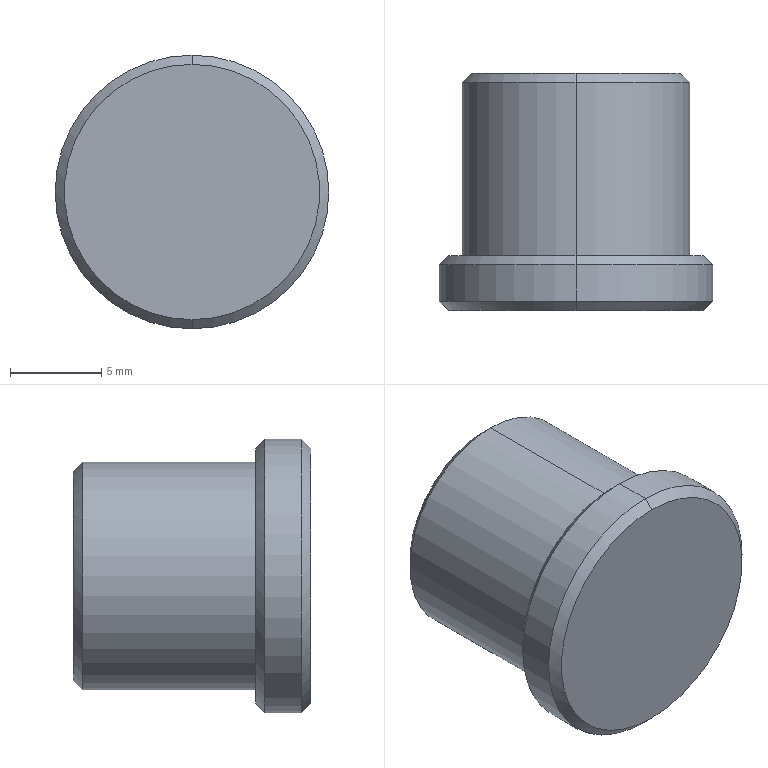Part | SolidWorks | features Chamfer 1, Revolution 1 | 1 solid | 13 faces | box 15 x 13 x 15 mm | volume 1741 mm3 | cone 6 | cylinder 4 | plane 3 | commonest cylinder face diameters 12.5 x2 15 x2
STEP:
#1=CARTESIAN_POINT('',(0.,13.,5.75));
#2=VERTEX_POINT('',#1);
#3=CARTESIAN_POINT('',(0.,13.,-5.75));
#4=VERTEX_POINT('',#3);
#5=CARTESIAN_POINT('',(0.,13.,0.));
#6=DIRECTION('',(0.,1.,0.));
#7=DIRECTION('',(0.,0.,1.));
#8=AXIS2_PLACEMENT_3D('',#5,#6,#7);
#9=CIRCLE('',#8,5.75);
#10=EDGE_CURVE('',#2,#4,#9,.T.);
#11=ORIENTED_EDGE('',*,*,#10,.F.);
#12=CARTESIAN_POINT('',(0.,12.5,6.25));
#13=VERTEX_POINT('',#12);
#14=CARTESIAN_POINT('',(0.,12.5,6.25));
#15=DIRECTION('',(0.,-0.7071,0.7071));
#16=VECTOR('',#15,1000.);
#17=LINE('',#14,#16);
#18=EDGE_CURVE('',#2,#13,#17,.T.);
#19=ORIENTED_EDGE('',*,*,#18,.T.);
#20=CARTESIAN_POINT('',(0.,12.5,-6.25));
#21=VERTEX_POINT('',#20);
#22=CARTESIAN_POINT('',(0.,12.5,0.));
#23=DIRECTION('',(0.,-1.,0.));
#24=DIRECTION('',(0.,0.,1.));
#25=AXIS2_PLACEMENT_3D('',#22,#23,#24);
#26=CIRCLE('',#25,6.25);
#27=EDGE_CURVE('',#21,#13,#26,.T.);
#28=ORIENTED_EDGE('',*,*,#27,.F.);
#29=CARTESIAN_POINT('',(0.,12.5,-6.25));
#30=DIRECTION('',(0.,-0.7071,-0.7071));
#31=VECTOR('',#30,1000.);
#32=LINE('',#29,#31);
#33=EDGE_CURVE('',#4,#21,#32,.T.);
#34=ORIENTED_EDGE('',*,*,#33,.F.);
#35=EDGE_LOOP('',(#11,#19,#28,#34));
#36=FACE_OUTER_BOUND('',#35,.T.);
#37=CARTESIAN_POINT('',(0.,12.5,0.));
#38=DIRECTION('',(0.,-1.,0.));
#39=DIRECTION('',(0.,0.,-1.));
#40=AXIS2_PLACEMENT_3D('',#37,#38,#39);
#41=CONICAL_SURFACE('',#40,6.25,0.7854);
#42=ADVANCED_FACE('',(#36),#41,.T.);
#43=CARTESIAN_POINT('',(0.,3.,7.));
#44=VERTEX_POINT('',#43);
#45=CARTESIAN_POINT('',(0.,3.,-7.));
#46=VERTEX_POINT('',#45);
#47=CARTESIAN_POINT('',(0.,3.,0.));
#48=DIRECTION('',(0.,1.,0.));
#49=DIRECTION('',(0.,0.,1.));
#50=AXIS2_PLACEMENT_3D('',#47,#48,#49);
#51=CIRCLE('',#50,7.);
#52=EDGE_CURVE('',#44,#46,#51,.T.);
#53=ORIENTED_EDGE('',*,*,#52,.F.);
#54=CARTESIAN_POINT('',(0.,2.5,7.5));
#55=VERTEX_POINT('',#54);
#56=CARTESIAN_POINT('',(0.,2.5,7.5));
#57=DIRECTION('',(0.,-0.7071,0.7071));
#58=VECTOR('',#57,1000.);
#59=LINE('',#56,#58);
#60=EDGE_CURVE('',#44,#55,#59,.T.);
#61=ORIENTED_EDGE('',*,*,#60,.T.);
#62=CARTESIAN_POINT('',(0.,2.5,-7.5));
#63=VERTEX_POINT('',#62);
#64=CARTESIAN_POINT('',(0.,2.5,0.));
#65=DIRECTION('',(0.,-1.,0.));
#66=DIRECTION('',(0.,0.,1.));
#67=AXIS2_PLACEMENT_3D('',#64,#65,#66);
#68=CIRCLE('',#67,7.5);
#69=EDGE_CURVE('',#63,#55,#68,.T.);
#70=ORIENTED_EDGE('',*,*,#69,.F.);
#71=CARTESIAN_POINT('',(0.,2.5,-7.5));
#72=DIRECTION('',(0.,-0.7071,-0.7071));
#73=VECTOR('',#72,1000.);
#74=LINE('',#71,#73);
#75=EDGE_CURVE('',#46,#63,#74,.T.);
#76=ORIENTED_EDGE('',*,*,#75,.F.);
#77=EDGE_LOOP('',(#53,#61,#70,#76));
#78=FACE_OUTER_BOUND('',#77,.T.);
#79=CARTESIAN_POINT('',(0.,2.5,0.));
#80=DIRECTION('',(0.,-1.,0.));
#81=DIRECTION('',(0.,0.,-1.));
#82=AXIS2_PLACEMENT_3D('',#79,#80,#81);
#83=CONICAL_SURFACE('',#82,7.5,0.7854);
#84=ADVANCED_FACE('',(#78),#83,.T.);
#85=CARTESIAN_POINT('',(0.,0.,-7.));
#86=VERTEX_POINT('',#85);
#87=CARTESIAN_POINT('',(0.,0.,7.));
#88=VERTEX_POINT('',#87);
#89=CARTESIAN_POINT('',(0.,0.,0.));
#90=DIRECTION('',(0.,-1.,0.));
#91=DIRECTION('',(0.,0.,-1.));
#92=AXIS2_PLACEMENT_3D('',#89,#90,#91);
#93=CIRCLE('',#92,7.);
#94=EDGE_CURVE('',#86,#88,#93,.T.);
#95=ORIENTED_EDGE('',*,*,#94,.F.);
#96=CARTESIAN_POINT('',(0.,0.5,-7.5));
#97=VERTEX_POINT('',#96);
#98=CARTESIAN_POINT('',(0.,0.,-7.));
#99=DIRECTION('',(0.,0.7071,-0.7071));
#100=VECTOR('',#99,1000.);
#101=LINE('',#98,#100);
#102=EDGE_CURVE('',#86,#97,#101,.T.);
#103=ORIENTED_EDGE('',*,*,#102,.T.);
#104=CARTESIAN_POINT('',(0.,0.5,7.5));
#105=VERTEX_POINT('',#104);
#106=CARTESIAN_POINT('',(0.,0.5,0.));
#107=DIRECTION('',(0.,1.,0.));
#108=DIRECTION('',(0.,0.,-1.));
#109=AXIS2_PLACEMENT_3D('',#106,#107,#108);
#110=CIRCLE('',#109,7.5);
#111=EDGE_CURVE('',#105,#97,#110,.T.);
#112=ORIENTED_EDGE('',*,*,#111,.F.);
#113=CARTESIAN_POINT('',(0.,0.,7.));
#114=DIRECTION('',(0.,0.7071,0.7071));
#115=VECTOR('',#114,1000.);
#116=LINE('',#113,#115);
#117=EDGE_CURVE('',#88,#105,#116,.T.);
#118=ORIENTED_EDGE('',*,*,#117,.F.);
#119=EDGE_LOOP('',(#95,#103,#112,#118));
#120=FACE_OUTER_BOUND('',#119,.T.);
#121=CARTESIAN_POINT('',(0.,0.,0.));
#122=DIRECTION('',(0.,1.,0.));
#123=DIRECTION('',(0.,0.,1.));
#124=AXIS2_PLACEMENT_3D('',#121,#122,#123);
#125=CONICAL_SURFACE('',#124,7.,0.7854);
#126=ADVANCED_FACE('',(#120),#125,.T.);
#127=ORIENTED_EDGE('',*,*,#69,.T.);
#128=CARTESIAN_POINT('',(0.,0.,7.5));
#129=DIRECTION('',(0.,-1.,0.));
#130=VECTOR('',#129,1000.);
#131=LINE('',#128,#130);
#132=EDGE_CURVE('',#55,#105,#131,.T.);
#133=ORIENTED_EDGE('',*,*,#132,.T.);
#134=ORIENTED_EDGE('',*,*,#111,.T.);
#135=CARTESIAN_POINT('',(0.,0.,-7.5));
#136=DIRECTION('',(0.,-1.,0.));
#137=VECTOR('',#136,1000.);
#138=LINE('',#135,#137);
#139=EDGE_CURVE('',#63,#97,#138,.T.);
#140=ORIENTED_EDGE('',*,*,#139,.F.);
#141=EDGE_LOOP('',(#127,#133,#134,#140));
#142=FACE_OUTER_BOUND('',#141,.T.);
#143=CARTESIAN_POINT('',(0.,0.,0.));
#144=DIRECTION('',(0.,-1.,0.));
#145=DIRECTION('',(0.,0.,-1.));
#146=AXIS2_PLACEMENT_3D('',#143,#144,#145);
#147=CYLINDRICAL_SURFACE('',#146,7.5);
#148=ADVANCED_FACE('',(#142),#147,.T.);
#149=ORIENTED_EDGE('',*,*,#27,.T.);
#150=CARTESIAN_POINT('',(0.,3.,6.25));
#151=VERTEX_POINT('',#150);
#152=CARTESIAN_POINT('',(0.,0.,6.25));
#153=DIRECTION('',(0.,-1.,0.));
#154=VECTOR('',#153,1000.);
#155=LINE('',#152,#154);
#156=EDGE_CURVE('',#13,#151,#155,.T.);
#157=ORIENTED_EDGE('',*,*,#156,.T.);
#158=CARTESIAN_POINT('',(0.,3.,-6.25));
#159=VERTEX_POINT('',#158);
#160=CARTESIAN_POINT('',(0.,3.,0.));
#161=DIRECTION('',(0.,-1.,0.));
#162=DIRECTION('',(0.,0.,-1.));
#163=AXIS2_PLACEMENT_3D('',#160,#161,#162);
#164=CIRCLE('',#163,6.25);
#165=EDGE_CURVE('',#159,#151,#164,.T.);
#166=ORIENTED_EDGE('',*,*,#165,.F.);
#167=CARTESIAN_POINT('',(0.,0.,-6.25));
#168=DIRECTION('',(0.,-1.,0.));
#169=VECTOR('',#168,1000.);
#170=LINE('',#167,#169);
#171=EDGE_CURVE('',#21,#159,#170,.T.);
#172=ORIENTED_EDGE('',*,*,#171,.F.);
#173=EDGE_LOOP('',(#149,#157,#166,#172));
#174=FACE_OUTER_BOUND('',#173,.T.);
#175=CARTESIAN_POINT('',(0.,0.,0.));
#176=DIRECTION('',(0.,-1.,0.));
#177=DIRECTION('',(0.,0.,-1.));
#178=AXIS2_PLACEMENT_3D('',#175,#176,#177);
#179=CYLINDRICAL_SURFACE('',#178,6.25);
#180=ADVANCED_FACE('',(#174),#179,.T.);
#181=CARTESIAN_POINT('',(0.,13.,0.));
#182=DIRECTION('',(0.,1.,0.));
#183=DIRECTION('',(0.,0.,1.));
#184=AXIS2_PLACEMENT_3D('',#181,#182,#183);
#185=CIRCLE('',#184,5.75);
#186=EDGE_CURVE('',#4,#2,#185,.T.);
#187=ORIENTED_EDGE('',*,*,#186,.T.);
#188=ORIENTED_EDGE('',*,*,#10,.T.);
#189=EDGE_LOOP('',(#187,#188));
#190=FACE_OUTER_BOUND('',#189,.T.);
#191=CARTESIAN_POINT('',(0.,13.,0.));
#192=DIRECTION('',(0.,1.,0.));
#193=DIRECTION('',(0.,0.,1.));
#194=AXIS2_PLACEMENT_3D('',#191,#192,#193);
#195=PLANE('',#194);
#196=ADVANCED_FACE('',(#190),#195,.T.);
#197=ORIENTED_EDGE('',*,*,#156,.F.);
#198=CARTESIAN_POINT('',(0.,12.5,0.));
#199=DIRECTION('',(0.,-1.,0.));
#200=DIRECTION('',(0.,0.,1.));
#201=AXIS2_PLACEMENT_3D('',#198,#199,#200);
#202=CIRCLE('',#201,6.25);
#203=EDGE_CURVE('',#13,#21,#202,.T.);
#204=ORIENTED_EDGE('',*,*,#203,.T.);
#205=ORIENTED_EDGE('',*,*,#171,.T.);
#206=CARTESIAN_POINT('',(0.,3.,0.));
#207=DIRECTION('',(0.,-1.,0.));
#208=DIRECTION('',(0.,0.,-1.));
#209=AXIS2_PLACEMENT_3D('',#206,#207,#208);
#210=CIRCLE('',#209,6.25);
#211=EDGE_CURVE('',#151,#159,#210,.T.);
#212=ORIENTED_EDGE('',*,*,#211,.F.);
#213=EDGE_LOOP('',(#197,#204,#205,#212));
#214=FACE_OUTER_BOUND('',#213,.T.);
#215=CARTESIAN_POINT('',(0.,0.,0.));
#216=DIRECTION('',(0.,-1.,0.));
#217=DIRECTION('',(0.,0.,-1.));
#218=AXIS2_PLACEMENT_3D('',#215,#216,#217);
#219=CYLINDRICAL_SURFACE('',#218,6.25);
#220=ADVANCED_FACE('',(#214),#219,.T.);
#221=CARTESIAN_POINT('',(0.,3.,0.));
#222=DIRECTION('',(0.,1.,0.));
#223=DIRECTION('',(0.,0.,1.));
#224=AXIS2_PLACEMENT_3D('',#221,#222,#223);
#225=CIRCLE('',#224,7.);
#226=EDGE_CURVE('',#46,#44,#225,.T.);
#227=ORIENTED_EDGE('',*,*,#226,.T.);
#228=ORIENTED_EDGE('',*,*,#52,.T.);
#229=EDGE_LOOP('',(#227,#228));
#230=FACE_OUTER_BOUND('',#229,.T.);
#231=ORIENTED_EDGE('',*,*,#165,.T.);
#232=ORIENTED_EDGE('',*,*,#211,.T.);
#233=EDGE_LOOP('',(#231,#232));
#234=FACE_BOUND('',#233,.T.);
#235=CARTESIAN_POINT('',(0.,3.,-6.25));
#236=DIRECTION('',(0.,1.,0.));
#237=DIRECTION('',(0.,0.,1.));
#238=AXIS2_PLACEMENT_3D('',#235,#236,#237);
#239=PLANE('',#238);
#240=ADVANCED_FACE('',(#230,#234),#239,.T.);
#241=ORIENTED_EDGE('',*,*,#132,.F.);
#242=CARTESIAN_POINT('',(0.,2.5,0.));
#243=DIRECTION('',(0.,-1.,0.));
#244=DIRECTION('',(0.,0.,1.));
#245=AXIS2_PLACEMENT_3D('',#242,#243,#244);
#246=CIRCLE('',#245,7.5);
#247=EDGE_CURVE('',#55,#63,#246,.T.);
#248=ORIENTED_EDGE('',*,*,#247,.T.);
#249=ORIENTED_EDGE('',*,*,#139,.T.);
#250=CARTESIAN_POINT('',(0.,0.5,0.));
#251=DIRECTION('',(0.,1.,0.));
#252=DIRECTION('',(0.,0.,-1.));
#253=AXIS2_PLACEMENT_3D('',#250,#251,#252);
#254=CIRCLE('',#253,7.5);
#255=EDGE_CURVE('',#97,#105,#254,.T.);
#256=ORIENTED_EDGE('',*,*,#255,.T.);
#257=EDGE_LOOP('',(#241,#248,#249,#256));
#258=FACE_OUTER_BOUND('',#257,.T.);
#259=CARTESIAN_POINT('',(0.,0.,0.));
#260=DIRECTION('',(0.,-1.,0.));
#261=DIRECTION('',(0.,0.,-1.));
#262=AXIS2_PLACEMENT_3D('',#259,#260,#261);
#263=CYLINDRICAL_SURFACE('',#262,7.5);
#264=ADVANCED_FACE('',(#258),#263,.T.);
#265=CARTESIAN_POINT('',(0.,0.,0.));
#266=DIRECTION('',(0.,-1.,0.));
#267=DIRECTION('',(0.,0.,-1.));
#268=AXIS2_PLACEMENT_3D('',#265,#266,#267);
#269=CIRCLE('',#268,7.);
#270=EDGE_CURVE('',#88,#86,#269,.T.);
#271=ORIENTED_EDGE('',*,*,#270,.T.);
#272=ORIENTED_EDGE('',*,*,#94,.T.);
#273=EDGE_LOOP('',(#271,#272));
#274=FACE_OUTER_BOUND('',#273,.T.);
#275=CARTESIAN_POINT('',(0.,0.,-7.5));
#276=DIRECTION('',(0.,-1.,0.));
#277=DIRECTION('',(0.,0.,-1.));
#278=AXIS2_PLACEMENT_3D('',#275,#276,#277);
#279=PLANE('',#278);
#280=ADVANCED_FACE('',(#274),#279,.T.);
#281=ORIENTED_EDGE('',*,*,#102,.F.);
#282=ORIENTED_EDGE('',*,*,#270,.F.);
#283=ORIENTED_EDGE('',*,*,#117,.T.);
#284=ORIENTED_EDGE('',*,*,#255,.F.);
#285=EDGE_LOOP('',(#281,#282,#283,#284));
#286=FACE_OUTER_BOUND('',#285,.T.);
#287=CARTESIAN_POINT('',(0.,0.,0.));
#288=DIRECTION('',(0.,1.,0.));
#289=DIRECTION('',(0.,0.,1.));
#290=AXIS2_PLACEMENT_3D('',#287,#288,#289);
#291=CONICAL_SURFACE('',#290,7.,0.7854);
#292=ADVANCED_FACE('',(#286),#291,.T.);
#293=ORIENTED_EDGE('',*,*,#60,.F.);
#294=ORIENTED_EDGE('',*,*,#226,.F.);
#295=ORIENTED_EDGE('',*,*,#75,.T.);
#296=ORIENTED_EDGE('',*,*,#247,.F.);
#297=EDGE_LOOP('',(#293,#294,#295,#296));
#298=FACE_OUTER_BOUND('',#297,.T.);
#299=CARTESIAN_POINT('',(0.,2.5,0.));
#300=DIRECTION('',(0.,-1.,0.));
#301=DIRECTION('',(0.,0.,-1.));
#302=AXIS2_PLACEMENT_3D('',#299,#300,#301);
#303=CONICAL_SURFACE('',#302,7.5,0.7854);
#304=ADVANCED_FACE('',(#298),#303,.T.);
#305=ORIENTED_EDGE('',*,*,#18,.F.);
#306=ORIENTED_EDGE('',*,*,#186,.F.);
#307=ORIENTED_EDGE('',*,*,#33,.T.);
#308=ORIENTED_EDGE('',*,*,#203,.F.);
#309=EDGE_LOOP('',(#305,#306,#307,#308));
#310=FACE_OUTER_BOUND('',#309,.T.);
#311=CARTESIAN_POINT('',(0.,12.5,0.));
#312=DIRECTION('',(0.,-1.,0.));
#313=DIRECTION('',(0.,0.,-1.));
#314=AXIS2_PLACEMENT_3D('',#311,#312,#313);
#315=CONICAL_SURFACE('',#314,6.25,0.7854);
#316=ADVANCED_FACE('',(#310),#315,.T.);
#317=CLOSED_SHELL('',(#42,#84,#126,#148,#180,#196,#220,#240,#264,#280,#292,#304,#316));
#318=MANIFOLD_SOLID_BREP('',#317);
#319=CARTESIAN_POINT('',(0.,0.,0.));
#320=DIRECTION('',(0.,0.,1.));
#321=DIRECTION('',(1.,0.,0.));
#322=AXIS2_PLACEMENT_3D('',#319,#320,#321);
#323=(LENGTH_UNIT()NAMED_UNIT(*)SI_UNIT(.MILLI.,.METRE.));
#324=UNCERTAINTY_MEASURE_WITH_UNIT(LENGTH_MEASURE(0.00001),#323,'','');
#325=(NAMED_UNIT(*)PLANE_ANGLE_UNIT()SI_UNIT($,.RADIAN.));
#326=(NAMED_UNIT(*)SI_UNIT($,.STERADIAN.)SOLID_ANGLE_UNIT());
#327=(GEOMETRIC_REPRESENTATION_CONTEXT(3)GLOBAL_UNCERTAINTY_ASSIGNED_CONTEXT((#324))GLOBAL_UNIT_ASSIGNED_CONTEXT((#323,#325,#326))REPRESENTATION_CONTEXT('',''));
#328=ADVANCED_BREP_SHAPE_REPRESENTATION('',(#318,#322),#327);